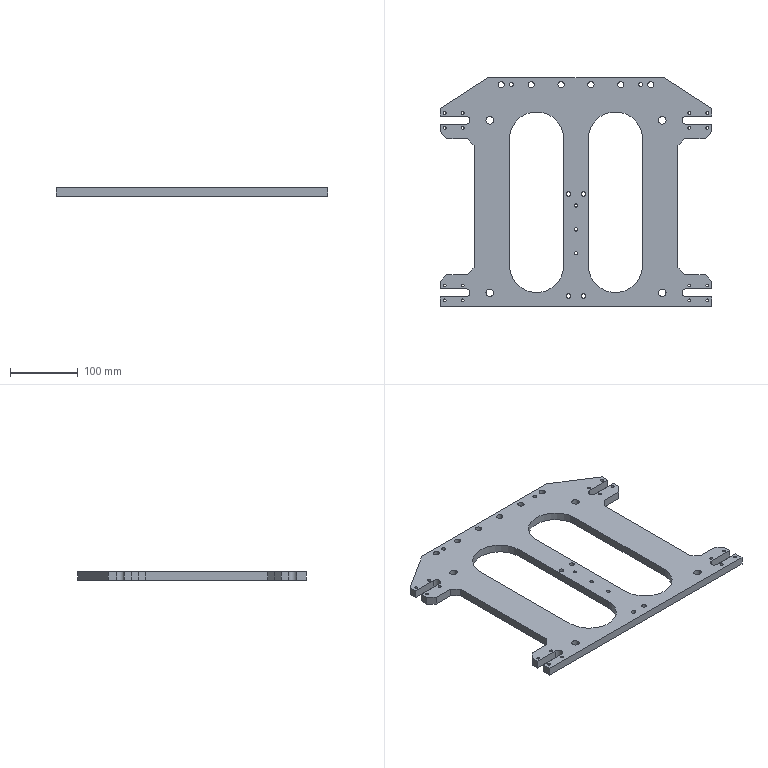CAM job | NX | 3-axis milling, drilling | part box 400 x 336 x 12 mm | stock box 404 x 340 x 12 mm
Tools:
number,name,description,diameter,corner_radius,flute_length,length,flutes
11,ZXZ,Milling Tool-5 Parameters,6.0,0.0,50.0,75.0,2
16,6.0ZT,Drilling Tool,6.0,0.0,35.0,50.0,2
19,9.0ZT,Drilling Tool,9.0,0.0,35.0,50.0,2
12,11.0ZT,Drilling Tool,11.0,0.0,35.0,50.0,2
10,D10,Milling Tool-5 Parameters,10.0,0.0,50.0,75.0,2
9,D10JING,Milling Tool-5 Parameters,10.0,0.0,50.0,75.0,2
6,D6,Milling Tool-5 Parameters,6.0,0.0,50.0,75.0,2
7,D6A45,Milling Tool-5 Parameters,6.0,0.0,3.0,3.0,2
14,4.2ZT,Drilling Tool,4.2,0.0,35.0,50.0,2
17,6.6ZT,Drilling Tool,6.6,0.0,35.0,50.0,2
15,5.0ZT,Drilling Tool,5.0,0.0,35.0,50.0,2
Operations:
program,operation,operation_type,tool,method,geometry_group,spindle_rpm,surface_speed,feed_per_tooth,feed_cut,feed_plunge,cut_length_mm,path_length_mm,cut_time_min,machine_time_min
1_CLAMP_LEFT_RIGHT,DRILLING,Operation,ZXZ,METHOD,A,3000.0,56.0,0.0417,250.0,0.0,140.0,2062.851,0.56,0.7523
1_CLAMP_LEFT_RIGHT,DRILLING_COPY,Operation,6.0ZT,METHOD,A,2000.0,37.0,0.045,180.0,0.0,36.605,426.234,0.2034,0.2423
1_CLAMP_LEFT_RIGHT,DRILLING_COPY_COPY_3,Operation,5.0ZT,METHOD,A,2000.0,37.0,0.045,180.0,0.0,54.007,344.27,0.3,0.3291
1_CLAMP_LEFT_RIGHT,DRILLING_COPY_COPY_2,Operation,6.6ZT,METHOD,A,2000.0,37.0,0.045,180.0,0.0,73.931,768.528,0.4107,0.4802
1_CLAMP_LEFT_RIGHT,DRILLING_COPY_COPY_1,Operation,4.2ZT,METHOD,A,2000.0,37.0,0.045,180.0,0.0,284.189,1855.534,1.579,1.736
1_CLAMP_LEFT_RIGHT,DRILLING_COPY_COPY,Operation,9.0ZT,METHOD,A,1000.0,28.0,0.09,180.0,0.0,115.223,625.957,0.6401,0.6912
1_CLAMP_LEFT_RIGHT,DRILLING_COPY_COPY_COPY,Operation,11.0ZT,METHOD,A,1000.0,28.0,0.09,180.0,0.0,79.219,1194.696,0.4401,0.5517
1_CLAMP_LEFT_RIGHT,ZLEVEL_PROFILE,ZLevelMilling,D10,METHOD,A,2200.0,69.0,0.5,2200.0,100.0,48855.802,49516.099,22.207,22.273
1_CLAMP_LEFT_RIGHT,ZLEVEL_PROFILE_COPY_1,ZLevelMilling,D10,METHOD,A,2200.0,69.0,0.5,2200.0,100.0,63918.708,64443.207,29.054,29.106
1_CLAMP_LEFT_RIGHT,ZLEVEL_PROFILE_COPY,ZLevelMilling,D10JING,METHOD,A,5000.0,157.0,0.12,1200.0,100.0,866.743,1529.529,0.7223,0.7886
1_CLAMP_LEFT_RIGHT,ZLEVEL_PROFILE_COPY_COPY_1,ZLevelMilling,D6,METHOD,A,5000.0,157.0,0.12,1200.0,100.0,1222.043,1843.445,1.018,1.081
1_CLAMP_LEFT_RIGHT,ZLEVEL_PROFILE_COPY_COPY,ZLevelMilling,D6A45,METHOD,A,7500.0,141.0,0.08,1200.0,100.0,2887.558,15746.094,2.406,3.692
2_CLAMP_FRONT_BACK,ZLEVEL_PROFILE_COPY_1_1,ZLevelMilling,D10,METHOD,A,2200.0,69.0,0.5,2200.0,100.0,61604.79,62380.345,28.002,28.08
2_CLAMP_FRONT_BACK,ZLEVEL_PROFILE_COPY_COPY_1_1,ZLevelMilling,D10JING,METHOD,A,5000.0,157.0,0.12,1200.0,100.0,1099.41,1874.381,0.9162,0.9937
2_CLAMP_FRONT_BACK,ZLEVEL_PROFILE_COPY_COPY_COPY,ZLevelMilling,D6A45,METHOD,A,7500.0,141.0,0.08,1200.0,100.0,1090.412,1806.226,0.9087,0.9803